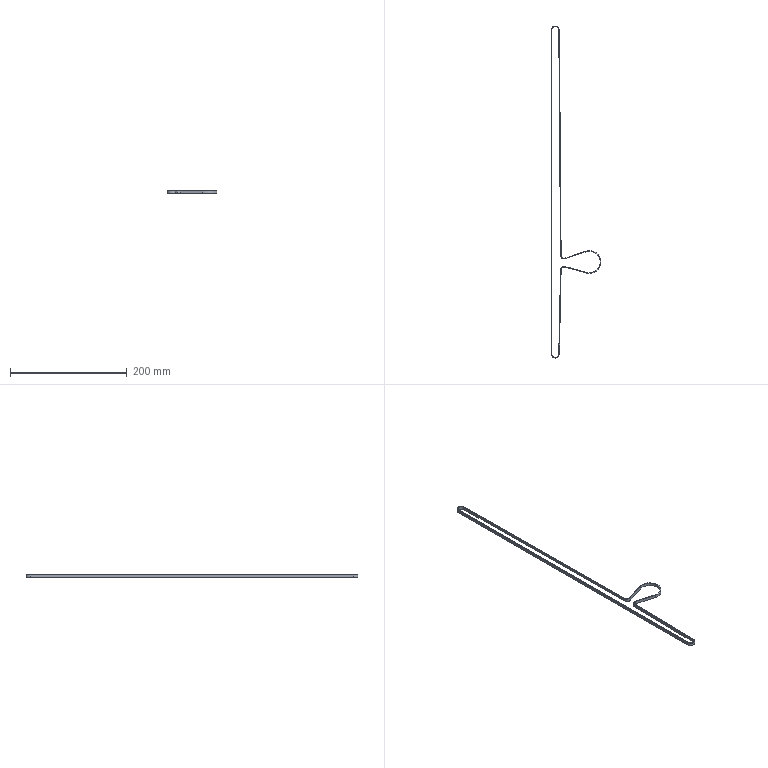Part | SolidWorks | features BaseBody 1 | 1 solid | 24 faces | box 85 x 569 x 5 mm | volume 6467 mm3 | cylinder 12 | plane 12 | commonest cylinder face diameters 12 x4 10 x2 14 x2 37 x2 39 x2
STEP:
#1=CARTESIAN_POINT('',(111.405,401.683,0.));
#2=VERTEX_POINT('',#1);
#3=CARTESIAN_POINT('',(135.678,384.107,0.));
#4=VERTEX_POINT('',#3);
#5=CARTESIAN_POINT('',(117.178,384.107,0.));
#6=DIRECTION('',(0.,0.,-1.));
#7=DIRECTION('',(1.,0.,0.));
#8=AXIS2_PLACEMENT_3D('',#5,#6,#7);
#9=CIRCLE('',#8,18.5);
#10=EDGE_CURVE('',#2,#4,#9,.T.);
#11=ORIENTED_EDGE('',*,*,#10,.T.);
#12=CARTESIAN_POINT('',(135.678,384.107,5.));
#13=VERTEX_POINT('',#12);
#14=CARTESIAN_POINT('',(135.678,384.107,0.));
#15=DIRECTION('',(0.,0.,1.));
#16=VECTOR('',#15,1000.);
#17=LINE('',#14,#16);
#18=EDGE_CURVE('',#4,#13,#17,.T.);
#19=ORIENTED_EDGE('',*,*,#18,.T.);
#20=CARTESIAN_POINT('',(111.405,401.683,5.));
#21=VERTEX_POINT('',#20);
#22=CARTESIAN_POINT('',(117.178,384.107,5.));
#23=DIRECTION('',(0.,0.,-1.));
#24=DIRECTION('',(1.,0.,0.));
#25=AXIS2_PLACEMENT_3D('',#22,#23,#24);
#26=CIRCLE('',#25,18.5);
#27=EDGE_CURVE('',#21,#13,#26,.T.);
#28=ORIENTED_EDGE('',*,*,#27,.F.);
#29=CARTESIAN_POINT('',(111.405,401.683,0.));
#30=DIRECTION('',(0.,0.,1.));
#31=VECTOR('',#30,1000.);
#32=LINE('',#29,#31);
#33=EDGE_CURVE('',#2,#21,#32,.T.);
#34=ORIENTED_EDGE('',*,*,#33,.F.);
#35=EDGE_LOOP('',(#11,#19,#28,#34));
#36=FACE_OUTER_BOUND('',#35,.T.);
#37=CARTESIAN_POINT('',(117.178,384.107,0.));
#38=DIRECTION('',(0.,0.,1.));
#39=DIRECTION('',(1.,0.,0.));
#40=AXIS2_PLACEMENT_3D('',#37,#38,#39);
#41=CYLINDRICAL_SURFACE('',#40,18.5);
#42=ADVANCED_FACE('',(#36),#41,.F.);
#43=CARTESIAN_POINT('',(112.033,365.298,0.));
#44=VERTEX_POINT('',#43);
#45=CARTESIAN_POINT('',(136.678,384.107,0.));
#46=VERTEX_POINT('',#45);
#47=CARTESIAN_POINT('',(117.178,384.107,0.));
#48=DIRECTION('',(0.,0.,1.));
#49=DIRECTION('',(1.,0.,0.));
#50=AXIS2_PLACEMENT_3D('',#47,#48,#49);
#51=CIRCLE('',#50,19.5);
#52=EDGE_CURVE('',#44,#46,#51,.T.);
#53=ORIENTED_EDGE('',*,*,#52,.T.);
#54=CARTESIAN_POINT('',(136.678,384.107,5.));
#55=VERTEX_POINT('',#54);
#56=CARTESIAN_POINT('',(136.678,384.107,0.));
#57=DIRECTION('',(0.,0.,1.));
#58=VECTOR('',#57,1000.);
#59=LINE('',#56,#58);
#60=EDGE_CURVE('',#46,#55,#59,.T.);
#61=ORIENTED_EDGE('',*,*,#60,.T.);
#62=CARTESIAN_POINT('',(112.033,365.298,5.));
#63=VERTEX_POINT('',#62);
#64=CARTESIAN_POINT('',(117.178,384.107,5.));
#65=DIRECTION('',(0.,0.,1.));
#66=DIRECTION('',(1.,0.,0.));
#67=AXIS2_PLACEMENT_3D('',#64,#65,#66);
#68=CIRCLE('',#67,19.5);
#69=EDGE_CURVE('',#63,#55,#68,.T.);
#70=ORIENTED_EDGE('',*,*,#69,.F.);
#71=CARTESIAN_POINT('',(112.033,365.298,0.));
#72=DIRECTION('',(0.,0.,-1.));
#73=VECTOR('',#72,1000.);
#74=LINE('',#71,#73);
#75=EDGE_CURVE('',#63,#44,#74,.T.);
#76=ORIENTED_EDGE('',*,*,#75,.T.);
#77=EDGE_LOOP('',(#53,#61,#70,#76));
#78=FACE_OUTER_BOUND('',#77,.T.);
#79=CARTESIAN_POINT('',(117.178,384.107,0.));
#80=DIRECTION('',(0.,0.,1.));
#81=DIRECTION('',(1.,0.,0.));
#82=AXIS2_PLACEMENT_3D('',#79,#80,#81);
#83=CYLINDRICAL_SURFACE('',#82,19.5);
#84=ADVANCED_FACE('',(#78),#83,.T.);
#85=CARTESIAN_POINT('',(52.678,226.607,0.));
#86=VERTEX_POINT('',#85);
#87=CARTESIAN_POINT('',(52.678,226.607,5.));
#88=VERTEX_POINT('',#87);
#89=CARTESIAN_POINT('',(52.678,226.607,0.));
#90=DIRECTION('',(0.,0.,1.));
#91=VECTOR('',#90,1000.);
#92=LINE('',#89,#91);
#93=EDGE_CURVE('',#86,#88,#92,.T.);
#94=ORIENTED_EDGE('',*,*,#93,.F.);
#95=CARTESIAN_POINT('',(52.678,781.607,0.));
#96=VERTEX_POINT('',#95);
#97=CARTESIAN_POINT('',(52.678,226.607,0.));
#98=DIRECTION('',(0.,-1.,0.));
#99=VECTOR('',#98,1000.);
#100=LINE('',#97,#99);
#101=EDGE_CURVE('',#96,#86,#100,.T.);
#102=ORIENTED_EDGE('',*,*,#101,.F.);
#103=CARTESIAN_POINT('',(52.678,781.607,5.));
#104=VERTEX_POINT('',#103);
#105=CARTESIAN_POINT('',(52.678,781.607,0.));
#106=DIRECTION('',(0.,0.,-1.));
#107=VECTOR('',#106,1000.);
#108=LINE('',#105,#107);
#109=EDGE_CURVE('',#104,#96,#108,.T.);
#110=ORIENTED_EDGE('',*,*,#109,.F.);
#111=CARTESIAN_POINT('',(52.678,226.607,5.));
#112=DIRECTION('',(0.,1.,0.));
#113=VECTOR('',#112,1000.);
#114=LINE('',#111,#113);
#115=EDGE_CURVE('',#88,#104,#114,.T.);
#116=ORIENTED_EDGE('',*,*,#115,.F.);
#117=EDGE_LOOP('',(#94,#102,#110,#116));
#118=FACE_OUTER_BOUND('',#117,.T.);
#119=CARTESIAN_POINT('',(52.678,226.607,0.));
#120=DIRECTION('',(-1.,0.,0.));
#121=DIRECTION('',(0.,0.,1.));
#122=AXIS2_PLACEMENT_3D('',#119,#120,#121);
#123=PLANE('',#122);
#124=ADVANCED_FACE('',(#118),#123,.F.);
#125=CARTESIAN_POINT('',(64.677,226.482,5.));
#126=VERTEX_POINT('',#125);
#127=CARTESIAN_POINT('',(58.678,226.607,5.));
#128=DIRECTION('',(0.,0.,-1.));
#129=DIRECTION('',(1.,0.,0.));
#130=AXIS2_PLACEMENT_3D('',#127,#128,#129);
#131=CIRCLE('',#130,6.);
#132=EDGE_CURVE('',#126,#88,#131,.T.);
#133=ORIENTED_EDGE('',*,*,#132,.T.);
#134=ORIENTED_EDGE('',*,*,#115,.T.);
#135=CARTESIAN_POINT('',(64.678,781.654,5.));
#136=VERTEX_POINT('',#135);
#137=CARTESIAN_POINT('',(58.678,781.607,5.));
#138=DIRECTION('',(0.,0.,-1.));
#139=DIRECTION('',(1.,0.,0.));
#140=AXIS2_PLACEMENT_3D('',#137,#138,#139);
#141=CIRCLE('',#140,6.);
#142=EDGE_CURVE('',#104,#136,#141,.T.);
#143=ORIENTED_EDGE('',*,*,#142,.T.);
#144=CARTESIAN_POINT('',(67.678,395.56,5.));
#145=VERTEX_POINT('',#144);
#146=CARTESIAN_POINT('',(64.678,781.654,5.));
#147=DIRECTION('',(0.007771,-1.,0.));
#148=VECTOR('',#147,1000.);
#149=LINE('',#146,#148);
#150=EDGE_CURVE('',#136,#145,#149,.T.);
#151=ORIENTED_EDGE('',*,*,#150,.T.);
#152=CARTESIAN_POINT('',(75.55,389.907,5.));
#153=VERTEX_POINT('',#152);
#154=CARTESIAN_POINT('',(73.678,395.607,5.));
#155=DIRECTION('',(0.,0.,1.));
#156=DIRECTION('',(1.,0.,0.));
#157=AXIS2_PLACEMENT_3D('',#154,#155,#156);
#158=CIRCLE('',#157,6.);
#159=EDGE_CURVE('',#145,#153,#158,.T.);
#160=ORIENTED_EDGE('',*,*,#159,.T.);
#161=CARTESIAN_POINT('',(75.55,389.907,5.));
#162=DIRECTION('',(0.9501,0.3121,0.));
#163=VECTOR('',#162,1000.);
#164=LINE('',#161,#163);
#165=EDGE_CURVE('',#153,#21,#164,.T.);
#166=ORIENTED_EDGE('',*,*,#165,.T.);
#167=ORIENTED_EDGE('',*,*,#27,.T.);
#168=CARTESIAN_POINT('',(112.297,366.263,5.));
#169=VERTEX_POINT('',#168);
#170=CARTESIAN_POINT('',(117.178,384.107,5.));
#171=DIRECTION('',(0.,0.,-1.));
#172=DIRECTION('',(1.,0.,0.));
#173=AXIS2_PLACEMENT_3D('',#170,#171,#172);
#174=CIRCLE('',#173,18.5);
#175=EDGE_CURVE('',#13,#169,#174,.T.);
#176=ORIENTED_EDGE('',*,*,#175,.T.);
#177=CARTESIAN_POINT('',(75.261,376.394,5.));
#178=VERTEX_POINT('',#177);
#179=CARTESIAN_POINT('',(112.297,366.263,5.));
#180=DIRECTION('',(-0.9646,0.2639,0.));
#181=VECTOR('',#180,1000.);
#182=LINE('',#179,#181);
#183=EDGE_CURVE('',#169,#178,#182,.T.);
#184=ORIENTED_EDGE('',*,*,#183,.T.);
#185=CARTESIAN_POINT('',(67.679,370.732,5.));
#186=VERTEX_POINT('',#185);
#187=CARTESIAN_POINT('',(73.678,370.607,5.));
#188=DIRECTION('',(0.,0.,1.));
#189=DIRECTION('',(1.,0.,0.));
#190=AXIS2_PLACEMENT_3D('',#187,#188,#189);
#191=CIRCLE('',#190,6.);
#192=EDGE_CURVE('',#178,#186,#191,.T.);
#193=ORIENTED_EDGE('',*,*,#192,.T.);
#194=CARTESIAN_POINT('',(67.679,370.732,5.));
#195=DIRECTION('',(-0.02081,-0.9998,0.));
#196=VECTOR('',#195,1000.);
#197=LINE('',#194,#196);
#198=EDGE_CURVE('',#186,#126,#197,.T.);
#199=ORIENTED_EDGE('',*,*,#198,.T.);
#200=EDGE_LOOP('',(#133,#134,#143,#151,#160,#166,#167,#176,#184,#193,#199));
#201=FACE_BOUND('',#200,.T.);
#202=CARTESIAN_POINT('',(75.238,390.857,5.));
#203=VERTEX_POINT('',#202);
#204=CARTESIAN_POINT('',(68.678,395.568,5.));
#205=VERTEX_POINT('',#204);
#206=CARTESIAN_POINT('',(73.678,395.607,5.));
#207=DIRECTION('',(0.,0.,-1.));
#208=DIRECTION('',(1.,0.,0.));
#209=AXIS2_PLACEMENT_3D('',#206,#207,#208);
#210=CIRCLE('',#209,5.);
#211=EDGE_CURVE('',#203,#205,#210,.T.);
#212=ORIENTED_EDGE('',*,*,#211,.T.);
#213=CARTESIAN_POINT('',(65.678,781.661,5.));
#214=VERTEX_POINT('',#213);
#215=CARTESIAN_POINT('',(68.678,395.568,5.));
#216=DIRECTION('',(-0.007771,1.,0.));
#217=VECTOR('',#216,1000.);
#218=LINE('',#215,#217);
#219=EDGE_CURVE('',#205,#214,#218,.T.);
#220=ORIENTED_EDGE('',*,*,#219,.T.);
#221=CARTESIAN_POINT('',(51.678,781.607,5.));
#222=VERTEX_POINT('',#221);
#223=CARTESIAN_POINT('',(58.678,781.607,5.));
#224=DIRECTION('',(0.,0.,1.));
#225=DIRECTION('',(1.,0.,0.));
#226=AXIS2_PLACEMENT_3D('',#223,#224,#225);
#227=CIRCLE('',#226,7.);
#228=EDGE_CURVE('',#214,#222,#227,.T.);
#229=ORIENTED_EDGE('',*,*,#228,.T.);
#230=CARTESIAN_POINT('',(51.678,226.607,5.));
#231=VERTEX_POINT('',#230);
#232=CARTESIAN_POINT('',(51.678,490.899,5.));
#233=DIRECTION('',(0.,-1.,0.));
#234=VECTOR('',#233,1000.);
#235=LINE('',#232,#234);
#236=EDGE_CURVE('',#222,#231,#235,.T.);
#237=ORIENTED_EDGE('',*,*,#236,.T.);
#238=CARTESIAN_POINT('',(65.677,226.461,5.));
#239=VERTEX_POINT('',#238);
#240=CARTESIAN_POINT('',(58.678,226.607,5.));
#241=DIRECTION('',(0.,0.,1.));
#242=DIRECTION('',(1.,0.,0.));
#243=AXIS2_PLACEMENT_3D('',#240,#241,#242);
#244=CIRCLE('',#243,7.);
#245=EDGE_CURVE('',#231,#239,#244,.T.);
#246=ORIENTED_EDGE('',*,*,#245,.T.);
#247=CARTESIAN_POINT('',(68.679,370.711,5.));
#248=VERTEX_POINT('',#247);
#249=CARTESIAN_POINT('',(65.677,226.461,5.));
#250=DIRECTION('',(0.02081,0.9998,0.));
#251=VECTOR('',#250,1000.);
#252=LINE('',#249,#251);
#253=EDGE_CURVE('',#239,#248,#252,.T.);
#254=ORIENTED_EDGE('',*,*,#253,.T.);
#255=CARTESIAN_POINT('',(74.998,375.43,5.));
#256=VERTEX_POINT('',#255);
#257=CARTESIAN_POINT('',(73.678,370.607,5.));
#258=DIRECTION('',(0.,0.,-1.));
#259=DIRECTION('',(1.,0.,0.));
#260=AXIS2_PLACEMENT_3D('',#257,#258,#259);
#261=CIRCLE('',#260,5.);
#262=EDGE_CURVE('',#248,#256,#261,.T.);
#263=ORIENTED_EDGE('',*,*,#262,.T.);
#264=CARTESIAN_POINT('',(74.998,375.43,5.));
#265=DIRECTION('',(0.9646,-0.2639,0.));
#266=VECTOR('',#265,1000.);
#267=LINE('',#264,#266);
#268=EDGE_CURVE('',#256,#63,#267,.T.);
#269=ORIENTED_EDGE('',*,*,#268,.T.);
#270=ORIENTED_EDGE('',*,*,#69,.T.);
#271=CARTESIAN_POINT('',(111.093,402.633,5.));
#272=VERTEX_POINT('',#271);
#273=CARTESIAN_POINT('',(117.178,384.107,5.));
#274=DIRECTION('',(0.,0.,1.));
#275=DIRECTION('',(1.,0.,0.));
#276=AXIS2_PLACEMENT_3D('',#273,#274,#275);
#277=CIRCLE('',#276,19.5);
#278=EDGE_CURVE('',#55,#272,#277,.T.);
#279=ORIENTED_EDGE('',*,*,#278,.T.);
#280=CARTESIAN_POINT('',(111.093,402.633,5.));
#281=DIRECTION('',(-0.9501,-0.3121,0.));
#282=VECTOR('',#281,1000.);
#283=LINE('',#280,#282);
#284=EDGE_CURVE('',#272,#203,#283,.T.);
#285=ORIENTED_EDGE('',*,*,#284,.T.);
#286=EDGE_LOOP('',(#212,#220,#229,#237,#246,#254,#263,#269,#270,#279,#285));
#287=FACE_OUTER_BOUND('',#286,.T.);
#288=CARTESIAN_POINT('',(65.127,490.899,5.));
#289=DIRECTION('',(0.,0.,1.));
#290=DIRECTION('',(1.,0.,0.));
#291=AXIS2_PLACEMENT_3D('',#288,#289,#290);
#292=PLANE('',#291);
#293=ADVANCED_FACE('',(#201,#287),#292,.T.);
#294=CARTESIAN_POINT('',(64.677,226.482,0.));
#295=VERTEX_POINT('',#294);
#296=CARTESIAN_POINT('',(64.677,226.482,0.));
#297=DIRECTION('',(0.,0.,1.));
#298=VECTOR('',#297,1000.);
#299=LINE('',#296,#298);
#300=EDGE_CURVE('',#295,#126,#299,.T.);
#301=ORIENTED_EDGE('',*,*,#300,.F.);
#302=CARTESIAN_POINT('',(58.678,226.607,0.));
#303=DIRECTION('',(0.,0.,1.));
#304=DIRECTION('',(1.,0.,0.));
#305=AXIS2_PLACEMENT_3D('',#302,#303,#304);
#306=CIRCLE('',#305,6.);
#307=EDGE_CURVE('',#86,#295,#306,.T.);
#308=ORIENTED_EDGE('',*,*,#307,.F.);
#309=ORIENTED_EDGE('',*,*,#93,.T.);
#310=ORIENTED_EDGE('',*,*,#132,.F.);
#311=EDGE_LOOP('',(#301,#308,#309,#310));
#312=FACE_OUTER_BOUND('',#311,.T.);
#313=CARTESIAN_POINT('',(58.678,226.607,0.));
#314=DIRECTION('',(0.,0.,1.));
#315=DIRECTION('',(1.,0.,0.));
#316=AXIS2_PLACEMENT_3D('',#313,#314,#315);
#317=CYLINDRICAL_SURFACE('',#316,6.);
#318=ADVANCED_FACE('',(#312),#317,.F.);
#319=ORIENTED_EDGE('',*,*,#101,.T.);
#320=ORIENTED_EDGE('',*,*,#307,.T.);
#321=CARTESIAN_POINT('',(67.679,370.732,0.));
#322=VERTEX_POINT('',#321);
#323=CARTESIAN_POINT('',(67.679,370.732,0.));
#324=DIRECTION('',(-0.02081,-0.9998,0.));
#325=VECTOR('',#324,1000.);
#326=LINE('',#323,#325);
#327=EDGE_CURVE('',#322,#295,#326,.T.);
#328=ORIENTED_EDGE('',*,*,#327,.F.);
#329=CARTESIAN_POINT('',(75.261,376.394,0.));
#330=VERTEX_POINT('',#329);
#331=CARTESIAN_POINT('',(73.678,370.607,0.));
#332=DIRECTION('',(0.,0.,1.));
#333=DIRECTION('',(1.,0.,0.));
#334=AXIS2_PLACEMENT_3D('',#331,#332,#333);
#335=CIRCLE('',#334,6.);
#336=EDGE_CURVE('',#330,#322,#335,.T.);
#337=ORIENTED_EDGE('',*,*,#336,.F.);
#338=CARTESIAN_POINT('',(112.297,366.263,0.));
#339=VERTEX_POINT('',#338);
#340=CARTESIAN_POINT('',(112.297,366.263,0.));
#341=DIRECTION('',(-0.9646,0.2639,0.));
#342=VECTOR('',#341,1000.);
#343=LINE('',#340,#342);
#344=EDGE_CURVE('',#339,#330,#343,.T.);
#345=ORIENTED_EDGE('',*,*,#344,.F.);
#346=CARTESIAN_POINT('',(117.178,384.107,0.));
#347=DIRECTION('',(0.,0.,-1.));
#348=DIRECTION('',(1.,0.,0.));
#349=AXIS2_PLACEMENT_3D('',#346,#347,#348);
#350=CIRCLE('',#349,18.5);
#351=EDGE_CURVE('',#4,#339,#350,.T.);
#352=ORIENTED_EDGE('',*,*,#351,.F.);
#353=ORIENTED_EDGE('',*,*,#10,.F.);
#354=CARTESIAN_POINT('',(75.55,389.907,0.));
#355=VERTEX_POINT('',#354);
#356=CARTESIAN_POINT('',(75.55,389.907,0.));
#357=DIRECTION('',(0.9501,0.3121,0.));
#358=VECTOR('',#357,1000.);
#359=LINE('',#356,#358);
#360=EDGE_CURVE('',#355,#2,#359,.T.);
#361=ORIENTED_EDGE('',*,*,#360,.F.);
#362=CARTESIAN_POINT('',(67.678,395.56,0.));
#363=VERTEX_POINT('',#362);
#364=CARTESIAN_POINT('',(73.678,395.607,0.));
#365=DIRECTION('',(0.,0.,1.));
#366=DIRECTION('',(1.,0.,0.));
#367=AXIS2_PLACEMENT_3D('',#364,#365,#366);
#368=CIRCLE('',#367,6.);
#369=EDGE_CURVE('',#363,#355,#368,.T.);
#370=ORIENTED_EDGE('',*,*,#369,.F.);
#371=CARTESIAN_POINT('',(64.678,781.654,0.));
#372=VERTEX_POINT('',#371);
#373=CARTESIAN_POINT('',(64.678,781.654,0.));
#374=DIRECTION('',(0.007771,-1.,0.));
#375=VECTOR('',#374,1000.);
#376=LINE('',#373,#375);
#377=EDGE_CURVE('',#372,#363,#376,.T.);
#378=ORIENTED_EDGE('',*,*,#377,.F.);
#379=CARTESIAN_POINT('',(58.678,781.607,0.));
#380=DIRECTION('',(0.,0.,-1.));
#381=DIRECTION('',(1.,0.,0.));
#382=AXIS2_PLACEMENT_3D('',#379,#380,#381);
#383=CIRCLE('',#382,6.);
#384=EDGE_CURVE('',#96,#372,#383,.T.);
#385=ORIENTED_EDGE('',*,*,#384,.F.);
#386=EDGE_LOOP('',(#319,#320,#328,#337,#345,#352,#353,#361,#370,#378,#385));
#387=FACE_BOUND('',#386,.T.);
#388=CARTESIAN_POINT('',(65.678,781.661,0.));
#389=VERTEX_POINT('',#388);
#390=CARTESIAN_POINT('',(51.678,781.607,0.));
#391=VERTEX_POINT('',#390);
#392=CARTESIAN_POINT('',(58.678,781.607,0.));
#393=DIRECTION('',(0.,0.,1.));
#394=DIRECTION('',(1.,0.,0.));
#395=AXIS2_PLACEMENT_3D('',#392,#393,#394);
#396=CIRCLE('',#395,7.);
#397=EDGE_CURVE('',#389,#391,#396,.T.);
#398=ORIENTED_EDGE('',*,*,#397,.F.);
#399=CARTESIAN_POINT('',(68.678,395.568,0.));
#400=VERTEX_POINT('',#399);
#401=CARTESIAN_POINT('',(68.678,395.568,0.));
#402=DIRECTION('',(-0.007771,1.,0.));
#403=VECTOR('',#402,1000.);
#404=LINE('',#401,#403);
#405=EDGE_CURVE('',#400,#389,#404,.T.);
#406=ORIENTED_EDGE('',*,*,#405,.F.);
#407=CARTESIAN_POINT('',(75.238,390.857,0.));
#408=VERTEX_POINT('',#407);
#409=CARTESIAN_POINT('',(73.678,395.607,0.));
#410=DIRECTION('',(0.,0.,-1.));
#411=DIRECTION('',(1.,0.,0.));
#412=AXIS2_PLACEMENT_3D('',#409,#410,#411);
#413=CIRCLE('',#412,5.);
#414=EDGE_CURVE('',#408,#400,#413,.T.);
#415=ORIENTED_EDGE('',*,*,#414,.F.);
#416=CARTESIAN_POINT('',(111.093,402.633,0.));
#417=VERTEX_POINT('',#416);
#418=CARTESIAN_POINT('',(111.093,402.633,0.));
#419=DIRECTION('',(-0.9501,-0.3121,0.));
#420=VECTOR('',#419,1000.);
#421=LINE('',#418,#420);
#422=EDGE_CURVE('',#417,#408,#421,.T.);
#423=ORIENTED_EDGE('',*,*,#422,.F.);
#424=CARTESIAN_POINT('',(117.178,384.107,0.));
#425=DIRECTION('',(0.,0.,1.));
#426=DIRECTION('',(1.,0.,0.));
#427=AXIS2_PLACEMENT_3D('',#424,#425,#426);
#428=CIRCLE('',#427,19.5);
#429=EDGE_CURVE('',#46,#417,#428,.T.);
#430=ORIENTED_EDGE('',*,*,#429,.F.);
#431=ORIENTED_EDGE('',*,*,#52,.F.);
#432=CARTESIAN_POINT('',(74.998,375.43,0.));
#433=VERTEX_POINT('',#432);
#434=CARTESIAN_POINT('',(74.998,375.43,0.));
#435=DIRECTION('',(0.9646,-0.2639,0.));
#436=VECTOR('',#435,1000.);
#437=LINE('',#434,#436);
#438=EDGE_CURVE('',#433,#44,#437,.T.);
#439=ORIENTED_EDGE('',*,*,#438,.F.);
#440=CARTESIAN_POINT('',(68.679,370.711,0.));
#441=VERTEX_POINT('',#440);
#442=CARTESIAN_POINT('',(73.678,370.607,0.));
#443=DIRECTION('',(0.,0.,-1.));
#444=DIRECTION('',(1.,0.,0.));
#445=AXIS2_PLACEMENT_3D('',#442,#443,#444);
#446=CIRCLE('',#445,5.);
#447=EDGE_CURVE('',#441,#433,#446,.T.);
#448=ORIENTED_EDGE('',*,*,#447,.F.);
#449=CARTESIAN_POINT('',(65.677,226.461,0.));
#450=VERTEX_POINT('',#449);
#451=CARTESIAN_POINT('',(65.677,226.461,0.));
#452=DIRECTION('',(0.02081,0.9998,0.));
#453=VECTOR('',#452,1000.);
#454=LINE('',#451,#453);
#455=EDGE_CURVE('',#450,#441,#454,.T.);
#456=ORIENTED_EDGE('',*,*,#455,.F.);
#457=CARTESIAN_POINT('',(51.678,226.607,0.));
#458=VERTEX_POINT('',#457);
#459=CARTESIAN_POINT('',(58.678,226.607,0.));
#460=DIRECTION('',(0.,0.,1.));
#461=DIRECTION('',(1.,0.,0.));
#462=AXIS2_PLACEMENT_3D('',#459,#460,#461);
#463=CIRCLE('',#462,7.);
#464=EDGE_CURVE('',#458,#450,#463,.T.);
#465=ORIENTED_EDGE('',*,*,#464,.F.);
#466=CARTESIAN_POINT('',(51.678,490.899,0.));
#467=DIRECTION('',(0.,-1.,0.));
#468=VECTOR('',#467,1000.);
#469=LINE('',#466,#468);
#470=EDGE_CURVE('',#391,#458,#469,.T.);
#471=ORIENTED_EDGE('',*,*,#470,.F.);
#472=EDGE_LOOP('',(#398,#406,#415,#423,#430,#431,#439,#448,#456,#465,#471));
#473=FACE_OUTER_BOUND('',#472,.T.);
#474=CARTESIAN_POINT('',(65.127,490.899,0.));
#475=DIRECTION('',(0.,0.,1.));
#476=DIRECTION('',(1.,0.,0.));
#477=AXIS2_PLACEMENT_3D('',#474,#475,#476);
#478=PLANE('',#477);
#479=ADVANCED_FACE('',(#387,#473),#478,.F.);
#480=ORIENTED_EDGE('',*,*,#109,.T.);
#481=ORIENTED_EDGE('',*,*,#384,.T.);
#482=CARTESIAN_POINT('',(64.678,781.654,0.));
#483=DIRECTION('',(0.,0.,-1.));
#484=VECTOR('',#483,1000.);
#485=LINE('',#482,#484);
#486=EDGE_CURVE('',#136,#372,#485,.T.);
#487=ORIENTED_EDGE('',*,*,#486,.F.);
#488=ORIENTED_EDGE('',*,*,#142,.F.);
#489=EDGE_LOOP('',(#480,#481,#487,#488));
#490=FACE_OUTER_BOUND('',#489,.T.);
#491=CARTESIAN_POINT('',(58.678,781.607,0.));
#492=DIRECTION('',(0.,0.,1.));
#493=DIRECTION('',(1.,0.,0.));
#494=AXIS2_PLACEMENT_3D('',#491,#492,#493);
#495=CYLINDRICAL_SURFACE('',#494,6.);
#496=ADVANCED_FACE('',(#490),#495,.F.);
#497=CARTESIAN_POINT('',(67.679,370.732,0.));
#498=DIRECTION('',(0.,0.,1.));
#499=VECTOR('',#498,1000.);
#500=LINE('',#497,#499);
#501=EDGE_CURVE('',#322,#186,#500,.T.);
#502=ORIENTED_EDGE('',*,*,#501,.F.);
#503=ORIENTED_EDGE('',*,*,#327,.T.);
#504=ORIENTED_EDGE('',*,*,#300,.T.);
#505=ORIENTED_EDGE('',*,*,#198,.F.);
#506=EDGE_LOOP('',(#502,#503,#504,#505));
#507=FACE_OUTER_BOUND('',#506,.T.);
#508=CARTESIAN_POINT('',(67.679,370.732,0.));
#509=DIRECTION('',(0.9998,-0.02081,0.));
#510=DIRECTION('',(0.02081,0.9998,0.));
#511=AXIS2_PLACEMENT_3D('',#508,#509,#510);
#512=PLANE('',#511);
#513=ADVANCED_FACE('',(#507),#512,.F.);
#514=ORIENTED_EDGE('',*,*,#336,.T.);
#515=ORIENTED_EDGE('',*,*,#501,.T.);
#516=ORIENTED_EDGE('',*,*,#192,.F.);
#517=CARTESIAN_POINT('',(75.261,376.394,0.));
#518=DIRECTION('',(0.,0.,-1.));
#519=VECTOR('',#518,1000.);
#520=LINE('',#517,#519);
#521=EDGE_CURVE('',#178,#330,#520,.T.);
#522=ORIENTED_EDGE('',*,*,#521,.T.);
#523=EDGE_LOOP('',(#514,#515,#516,#522));
#524=FACE_OUTER_BOUND('',#523,.T.);
#525=CARTESIAN_POINT('',(73.678,370.607,0.));
#526=DIRECTION('',(0.,0.,1.));
#527=DIRECTION('',(1.,0.,0.));
#528=AXIS2_PLACEMENT_3D('',#525,#526,#527);
#529=CYLINDRICAL_SURFACE('',#528,6.);
#530=ADVANCED_FACE('',(#524),#529,.T.);
#531=CARTESIAN_POINT('',(112.297,366.263,0.));
#532=DIRECTION('',(0.,0.,1.));
#533=VECTOR('',#532,1000.);
#534=LINE('',#531,#533);
#535=EDGE_CURVE('',#339,#169,#534,.T.);
#536=ORIENTED_EDGE('',*,*,#535,.F.);
#537=ORIENTED_EDGE('',*,*,#344,.T.);
#538=ORIENTED_EDGE('',*,*,#521,.F.);
#539=ORIENTED_EDGE('',*,*,#183,.F.);
#540=EDGE_LOOP('',(#536,#537,#538,#539));
#541=FACE_OUTER_BOUND('',#540,.T.);
#542=CARTESIAN_POINT('',(112.297,366.263,0.));
#543=DIRECTION('',(-0.2639,-0.9646,0.));
#544=DIRECTION('',(0.9646,-0.2639,0.));
#545=AXIS2_PLACEMENT_3D('',#542,#543,#544);
#546=PLANE('',#545);
#547=ADVANCED_FACE('',(#541),#546,.F.);
#548=ORIENTED_EDGE('',*,*,#18,.F.);
#549=ORIENTED_EDGE('',*,*,#351,.T.);
#550=ORIENTED_EDGE('',*,*,#535,.T.);
#551=ORIENTED_EDGE('',*,*,#175,.F.);
#552=EDGE_LOOP('',(#548,#549,#550,#551));
#553=FACE_OUTER_BOUND('',#552,.T.);
#554=CARTESIAN_POINT('',(117.178,384.107,0.));
#555=DIRECTION('',(0.,0.,1.));
#556=DIRECTION('',(1.,0.,0.));
#557=AXIS2_PLACEMENT_3D('',#554,#555,#556);
#558=CYLINDRICAL_SURFACE('',#557,18.5);
#559=ADVANCED_FACE('',(#553),#558,.F.);
#560=CARTESIAN_POINT('',(75.55,389.907,0.));
#561=DIRECTION('',(0.,0.,1.));
#562=VECTOR('',#561,1000.);
#563=LINE('',#560,#562);
#564=EDGE_CURVE('',#355,#153,#563,.T.);
#565=ORIENTED_EDGE('',*,*,#564,.F.);
#566=ORIENTED_EDGE('',*,*,#360,.T.);
#567=ORIENTED_EDGE('',*,*,#33,.T.);
#568=ORIENTED_EDGE('',*,*,#165,.F.);
#569=EDGE_LOOP('',(#565,#566,#567,#568));
#570=FACE_OUTER_BOUND('',#569,.T.);
#571=CARTESIAN_POINT('',(75.55,389.907,0.));
#572=DIRECTION('',(-0.3121,0.9501,0.));
#573=DIRECTION('',(-0.9501,-0.3121,0.));
#574=AXIS2_PLACEMENT_3D('',#571,#572,#573);
#575=PLANE('',#574);
#576=ADVANCED_FACE('',(#570),#575,.F.);
#577=ORIENTED_EDGE('',*,*,#369,.T.);
#578=ORIENTED_EDGE('',*,*,#564,.T.);
#579=ORIENTED_EDGE('',*,*,#159,.F.);
#580=CARTESIAN_POINT('',(67.678,395.56,0.));
#581=DIRECTION('',(0.,0.,-1.));
#582=VECTOR('',#581,1000.);
#583=LINE('',#580,#582);
#584=EDGE_CURVE('',#145,#363,#583,.T.);
#585=ORIENTED_EDGE('',*,*,#584,.T.);
#586=EDGE_LOOP('',(#577,#578,#579,#585));
#587=FACE_OUTER_BOUND('',#586,.T.);
#588=CARTESIAN_POINT('',(73.678,395.607,0.));
#589=DIRECTION('',(0.,0.,1.));
#590=DIRECTION('',(1.,0.,0.));
#591=AXIS2_PLACEMENT_3D('',#588,#589,#590);
#592=CYLINDRICAL_SURFACE('',#591,6.);
#593=ADVANCED_FACE('',(#587),#592,.T.);
#594=ORIENTED_EDGE('',*,*,#486,.T.);
#595=ORIENTED_EDGE('',*,*,#377,.T.);
#596=ORIENTED_EDGE('',*,*,#584,.F.);
#597=ORIENTED_EDGE('',*,*,#150,.F.);
#598=EDGE_LOOP('',(#594,#595,#596,#597));
#599=FACE_OUTER_BOUND('',#598,.T.);
#600=CARTESIAN_POINT('',(64.678,781.654,0.));
#601=DIRECTION('',(1.,0.007771,0.));
#602=DIRECTION('',(-0.007771,1.,0.));
#603=AXIS2_PLACEMENT_3D('',#600,#601,#602);
#604=PLANE('',#603);
#605=ADVANCED_FACE('',(#599),#604,.F.);
#606=ORIENTED_EDGE('',*,*,#405,.T.);
#607=CARTESIAN_POINT('',(65.678,781.661,0.));
#608=DIRECTION('',(0.,0.,1.));
#609=VECTOR('',#608,1000.);
#610=LINE('',#607,#609);
#611=EDGE_CURVE('',#389,#214,#610,.T.);
#612=ORIENTED_EDGE('',*,*,#611,.T.);
#613=ORIENTED_EDGE('',*,*,#219,.F.);
#614=CARTESIAN_POINT('',(68.678,395.568,0.));
#615=DIRECTION('',(0.,0.,-1.));
#616=VECTOR('',#615,1000.);
#617=LINE('',#614,#616);
#618=EDGE_CURVE('',#205,#400,#617,.T.);
#619=ORIENTED_EDGE('',*,*,#618,.T.);
#620=EDGE_LOOP('',(#606,#612,#613,#619));
#621=FACE_OUTER_BOUND('',#620,.T.);
#622=CARTESIAN_POINT('',(65.678,781.661,0.));
#623=DIRECTION('',(1.,0.007771,0.));
#624=DIRECTION('',(-0.007771,1.,0.));
#625=AXIS2_PLACEMENT_3D('',#622,#623,#624);
#626=PLANE('',#625);
#627=ADVANCED_FACE('',(#621),#626,.T.);
#628=CARTESIAN_POINT('',(75.238,390.857,0.));
#629=DIRECTION('',(0.,0.,1.));
#630=VECTOR('',#629,1000.);
#631=LINE('',#628,#630);
#632=EDGE_CURVE('',#408,#203,#631,.T.);
#633=ORIENTED_EDGE('',*,*,#632,.F.);
#634=ORIENTED_EDGE('',*,*,#414,.T.);
#635=ORIENTED_EDGE('',*,*,#618,.F.);
#636=ORIENTED_EDGE('',*,*,#211,.F.);
#637=EDGE_LOOP('',(#633,#634,#635,#636));
#638=FACE_OUTER_BOUND('',#637,.T.);
#639=CARTESIAN_POINT('',(73.678,395.607,0.));
#640=DIRECTION('',(0.,0.,1.));
#641=DIRECTION('',(1.,0.,0.));
#642=AXIS2_PLACEMENT_3D('',#639,#640,#641);
#643=CYLINDRICAL_SURFACE('',#642,5.);
#644=ADVANCED_FACE('',(#638),#643,.F.);
#645=ORIENTED_EDGE('',*,*,#422,.T.);
#646=ORIENTED_EDGE('',*,*,#632,.T.);
#647=ORIENTED_EDGE('',*,*,#284,.F.);
#648=CARTESIAN_POINT('',(111.093,402.633,0.));
#649=DIRECTION('',(0.,0.,-1.));
#650=VECTOR('',#649,1000.);
#651=LINE('',#648,#650);
#652=EDGE_CURVE('',#272,#417,#651,.T.);
#653=ORIENTED_EDGE('',*,*,#652,.T.);
#654=EDGE_LOOP('',(#645,#646,#647,#653));
#655=FACE_OUTER_BOUND('',#654,.T.);
#656=CARTESIAN_POINT('',(75.238,390.857,0.));
#657=DIRECTION('',(-0.3121,0.9501,0.));
#658=DIRECTION('',(-0.9501,-0.3121,0.));
#659=AXIS2_PLACEMENT_3D('',#656,#657,#658);
#660=PLANE('',#659);
#661=ADVANCED_FACE('',(#655),#660,.T.);
#662=ORIENTED_EDGE('',*,*,#60,.F.);
#663=ORIENTED_EDGE('',*,*,#429,.T.);
#664=ORIENTED_EDGE('',*,*,#652,.F.);
#665=ORIENTED_EDGE('',*,*,#278,.F.);
#666=EDGE_LOOP('',(#662,#663,#664,#665));
#667=FACE_OUTER_BOUND('',#666,.T.);
#668=CARTESIAN_POINT('',(117.178,384.107,0.));
#669=DIRECTION('',(0.,0.,1.));
#670=DIRECTION('',(1.,0.,0.));
#671=AXIS2_PLACEMENT_3D('',#668,#669,#670);
#672=CYLINDRICAL_SURFACE('',#671,19.5);
#673=ADVANCED_FACE('',(#667),#672,.T.);
#674=ORIENTED_EDGE('',*,*,#438,.T.);
#675=ORIENTED_EDGE('',*,*,#75,.F.);
#676=ORIENTED_EDGE('',*,*,#268,.F.);
#677=CARTESIAN_POINT('',(74.998,375.43,0.));
#678=DIRECTION('',(0.,0.,-1.));
#679=VECTOR('',#678,1000.);
#680=LINE('',#677,#679);
#681=EDGE_CURVE('',#256,#433,#680,.T.);
#682=ORIENTED_EDGE('',*,*,#681,.T.);
#683=EDGE_LOOP('',(#674,#675,#676,#682));
#684=FACE_OUTER_BOUND('',#683,.T.);
#685=CARTESIAN_POINT('',(112.033,365.298,0.));
#686=DIRECTION('',(-0.2639,-0.9646,0.));
#687=DIRECTION('',(0.9646,-0.2639,0.));
#688=AXIS2_PLACEMENT_3D('',#685,#686,#687);
#689=PLANE('',#688);
#690=ADVANCED_FACE('',(#684),#689,.T.);
#691=CARTESIAN_POINT('',(68.679,370.711,0.));
#692=DIRECTION('',(0.,0.,1.));
#693=VECTOR('',#692,1000.);
#694=LINE('',#691,#693);
#695=EDGE_CURVE('',#441,#248,#694,.T.);
#696=ORIENTED_EDGE('',*,*,#695,.F.);
#697=ORIENTED_EDGE('',*,*,#447,.T.);
#698=ORIENTED_EDGE('',*,*,#681,.F.);
#699=ORIENTED_EDGE('',*,*,#262,.F.);
#700=EDGE_LOOP('',(#696,#697,#698,#699));
#701=FACE_OUTER_BOUND('',#700,.T.);
#702=CARTESIAN_POINT('',(73.678,370.607,0.));
#703=DIRECTION('',(0.,0.,1.));
#704=DIRECTION('',(1.,0.,0.));
#705=AXIS2_PLACEMENT_3D('',#702,#703,#704);
#706=CYLINDRICAL_SURFACE('',#705,5.);
#707=ADVANCED_FACE('',(#701),#706,.F.);
#708=ORIENTED_EDGE('',*,*,#455,.T.);
#709=ORIENTED_EDGE('',*,*,#695,.T.);
#710=ORIENTED_EDGE('',*,*,#253,.F.);
#711=CARTESIAN_POINT('',(65.677,226.461,0.));
#712=DIRECTION('',(0.,0.,-1.));
#713=VECTOR('',#712,1000.);
#714=LINE('',#711,#713);
#715=EDGE_CURVE('',#239,#450,#714,.T.);
#716=ORIENTED_EDGE('',*,*,#715,.T.);
#717=EDGE_LOOP('',(#708,#709,#710,#716));
#718=FACE_OUTER_BOUND('',#717,.T.);
#719=CARTESIAN_POINT('',(68.679,370.711,0.));
#720=DIRECTION('',(0.9998,-0.02081,0.));
#721=DIRECTION('',(0.02081,0.9998,0.));
#722=AXIS2_PLACEMENT_3D('',#719,#720,#721);
#723=PLANE('',#722);
#724=ADVANCED_FACE('',(#718),#723,.T.);
#725=ORIENTED_EDGE('',*,*,#464,.T.);
#726=ORIENTED_EDGE('',*,*,#715,.F.);
#727=ORIENTED_EDGE('',*,*,#245,.F.);
#728=CARTESIAN_POINT('',(51.678,226.607,0.));
#729=DIRECTION('',(0.,0.,-1.));
#730=VECTOR('',#729,1000.);
#731=LINE('',#728,#730);
#732=EDGE_CURVE('',#231,#458,#731,.T.);
#733=ORIENTED_EDGE('',*,*,#732,.T.);
#734=EDGE_LOOP('',(#725,#726,#727,#733));
#735=FACE_OUTER_BOUND('',#734,.T.);
#736=CARTESIAN_POINT('',(58.678,226.607,0.));
#737=DIRECTION('',(0.,0.,1.));
#738=DIRECTION('',(1.,0.,0.));
#739=AXIS2_PLACEMENT_3D('',#736,#737,#738);
#740=CYLINDRICAL_SURFACE('',#739,7.);
#741=ADVANCED_FACE('',(#735),#740,.T.);
#742=ORIENTED_EDGE('',*,*,#470,.T.);
#743=ORIENTED_EDGE('',*,*,#732,.F.);
#744=ORIENTED_EDGE('',*,*,#236,.F.);
#745=CARTESIAN_POINT('',(51.678,781.607,0.));
#746=DIRECTION('',(0.,0.,-1.));
#747=VECTOR('',#746,1000.);
#748=LINE('',#745,#747);
#749=EDGE_CURVE('',#222,#391,#748,.T.);
#750=ORIENTED_EDGE('',*,*,#749,.T.);
#751=EDGE_LOOP('',(#742,#743,#744,#750));
#752=FACE_OUTER_BOUND('',#751,.T.);
#753=CARTESIAN_POINT('',(51.678,226.607,0.));
#754=DIRECTION('',(-1.,0.,0.));
#755=DIRECTION('',(0.,0.,1.));
#756=AXIS2_PLACEMENT_3D('',#753,#754,#755);
#757=PLANE('',#756);
#758=ADVANCED_FACE('',(#752),#757,.T.);
#759=ORIENTED_EDGE('',*,*,#397,.T.);
#760=ORIENTED_EDGE('',*,*,#749,.F.);
#761=ORIENTED_EDGE('',*,*,#228,.F.);
#762=ORIENTED_EDGE('',*,*,#611,.F.);
#763=EDGE_LOOP('',(#759,#760,#761,#762));
#764=FACE_OUTER_BOUND('',#763,.T.);
#765=CARTESIAN_POINT('',(58.678,781.607,0.));
#766=DIRECTION('',(0.,0.,1.));
#767=DIRECTION('',(1.,0.,0.));
#768=AXIS2_PLACEMENT_3D('',#765,#766,#767);
#769=CYLINDRICAL_SURFACE('',#768,7.);
#770=ADVANCED_FACE('',(#764),#769,.T.);
#771=CLOSED_SHELL('',(#42,#84,#124,#293,#318,#479,#496,#513,#530,#547,#559,#576,#593,#605,#627,#644,#661,#673,#690,#707,#724,#741,#758,#770));
#772=MANIFOLD_SOLID_BREP('',#771);
#773=CARTESIAN_POINT('',(0.,0.,0.));
#774=DIRECTION('',(0.,0.,1.));
#775=DIRECTION('',(1.,0.,0.));
#776=AXIS2_PLACEMENT_3D('',#773,#774,#775);
#777=(LENGTH_UNIT()NAMED_UNIT(*)SI_UNIT(.MILLI.,.METRE.));
#778=UNCERTAINTY_MEASURE_WITH_UNIT(LENGTH_MEASURE(0.00001),#777,'','');
#779=(NAMED_UNIT(*)PLANE_ANGLE_UNIT()SI_UNIT($,.RADIAN.));
#780=(NAMED_UNIT(*)SI_UNIT($,.STERADIAN.)SOLID_ANGLE_UNIT());
#781=(GEOMETRIC_REPRESENTATION_CONTEXT(3)GLOBAL_UNCERTAINTY_ASSIGNED_CONTEXT((#778))GLOBAL_UNIT_ASSIGNED_CONTEXT((#777,#779,#780))REPRESENTATION_CONTEXT('',''));
#782=ADVANCED_BREP_SHAPE_REPRESENTATION('',(#772,#776),#781);